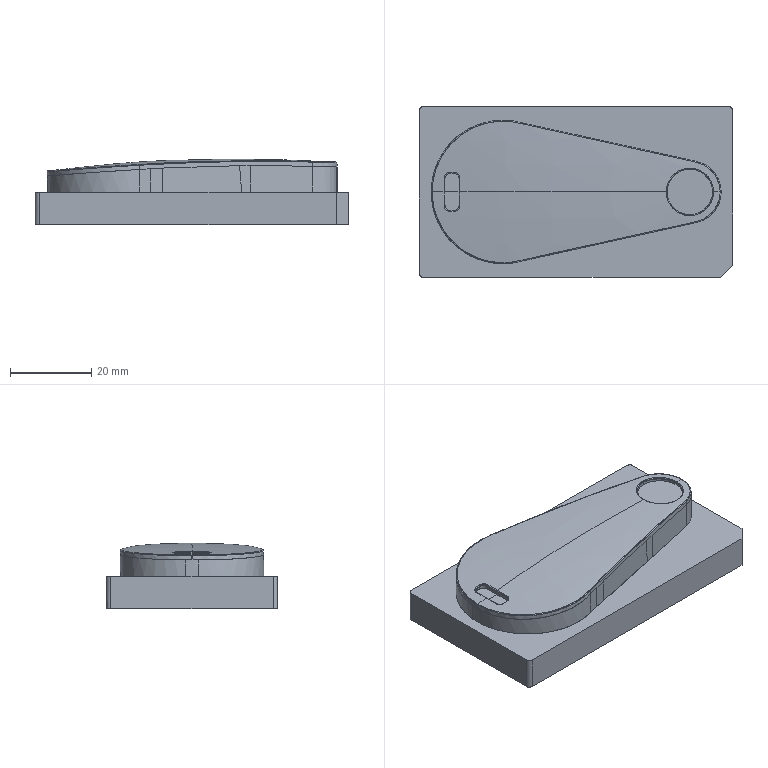NC program | PowerMill | posted with a generic post | part box 77 x 42 x 16.114 mm
Lines 19133 to 19848 of 230441:
N19230 M6
N19231 S18000 M03
N19232 G00 G90 X0.0 Y0.0
N19233 G43 Z10.803 H7
N19234
N19235 G05 P10000 R8
N19236 X35.209 Y-6.2591
N19237 Z-1.6006
N19238 G01 Z-2.8006 F1200.0
N19239 X35.1832 Y-6.2849 Z-2.7731 F2000.0
N19240 X35.1632 Y-6.3049 Z-2.7589
N19241 X35.1188 Y-6.3493 Z-2.7306
N19242 X35.0729 Y-6.3952 Z-2.7057
N19243 X35.0249 Y-6.4432 Z-2.6838
N19244 X34.9746 Y-6.4935 Z-2.6649
N19245 X34.9217 Y-6.5464 Z-2.6492
N19246 X34.8658 Y-6.6023 Z-2.6366
N19247 X34.8065 Y-6.6616 Z-2.6271
N19248 X34.772 Y-6.6961 Z-2.6234
N19249 X34.7334 Y-6.7347 Z-2.6213
N19250 X34.6899 Y-6.7782 Z-2.6212
N19251 X34.641 Y-6.8271 Z-2.6235
N19252 X34.5867 Y-6.8814 Z-2.6292
N19253 X34.5286 Y-6.9395 Z-2.6389
N19254 X34.4736 Y-6.9945 Z-2.6518
N19255 X34.4234 Y-7.0447 Z-2.6671
N19256 X34.3781 Y-7.09 Z-2.6843
N19257 X34.3373 Y-7.1308 Z-2.7032
N19258 X34.3008 Y-7.1673 Z-2.7235
N19259 X34.2682 Y-7.1999 Z-2.7452
N19260 X34.2385 Y-7.2296 Z-2.7686
N19261 X34.2146 Y-7.2535 Z-2.7954
N19262 X33.8245 Y-7.5729 Z-2.7981
N19263 X33.8519 Y-7.5454 Z-2.7464
N19264 X33.8774 Y-7.52 Z-2.7145
N19265 X33.9039 Y-7.4935 Z-2.6845
N19266 X33.9315 Y-7.4659 Z-2.6565
N19267 X33.9608 Y-7.4366 Z-2.6306
N19268 X33.9951 Y-7.4023 Z-2.6044
N19269 X34.031 Y-7.3663 Z-2.5806
N19270 X34.0646 Y-7.3327 Z-2.5605
N19271 X34.0976 Y-7.2998 Z-2.5418
N19272 X34.1447 Y-7.2527 Z-2.5181
N19273 X34.1959 Y-7.2015 Z-2.4964
N19274 X34.2517 Y-7.1457 Z-2.4768
N19275 X34.3126 Y-7.0848 Z-2.4593
N19276 X34.3735 Y-7.0238 Z-2.4452
N19277 X34.4416 Y-6.9558 Z-2.4327
N19278 X34.5099 Y-6.8875 Z-2.4237
N19279 X34.5798 Y-6.8176 Z-2.4182
N19280 X34.6486 Y-6.7487 Z-2.4166
N19281 X34.7173 Y-6.6801 Z-2.4183
N19282 X34.7812 Y-6.6162 Z-2.4228
N19283 X34.8542 Y-6.5432 Z-2.4313
N19284 X34.9245 Y-6.4729 Z-2.4434
N19285 X34.9922 Y-6.4052 Z-2.4588
N19286 X35.0574 Y-6.34 Z-2.4775
N19287 X35.1203 Y-6.2771 Z-2.4995
N19288 X35.1767 Y-6.2207 Z-2.5227
N19289 X35.2302 Y-6.1672 Z-2.5473
N19290 X35.2794 Y-6.1179 Z-2.5733
N19291 X35.3244 Y-6.073 Z-2.6006
N19292 X35.3656 Y-6.0318 Z-2.6297
N19293 X35.4036 Y-5.9938 Z-2.6606
N19294 X35.439 Y-5.9584 Z-2.6936
N19295 X35.4722 Y-5.9251 Z-2.7287
N19296 X35.5037 Y-5.8937 Z-2.7662
N19297 X35.5144 Y-5.8829 Z-2.78
N19298 X35.5428 Y-5.8546 Z-2.8245
N19299 X35.7727 Y-5.554 Z-2.8919
N19300 X35.7671 Y-5.5595 Z-2.869
N19301 X35.7378 Y-5.5889 Z-2.8034
N19302 X35.6641 Y-5.6625 Z-2.6896
N19303 X35.6342 Y-5.6924 Z-2.6536
N19304 X35.6006 Y-5.726 Z-2.6181
N19305 X35.563 Y-5.7637 Z-2.583
N19306 X35.5208 Y-5.8058 Z-2.5483
N19307 X35.4739 Y-5.8527 Z-2.5139
N19308 X35.4221 Y-5.9046 Z-2.4803
N19309 X35.366 Y-5.9607 Z-2.4481
N19310 X35.3094 Y-6.0173 Z-2.4194
N19311 X35.2572 Y-6.0695 Z-2.3958
N19312 X35.2101 Y-6.1165 Z-2.3768
N19313 X35.1703 Y-6.1564 Z-2.3621
N19314 X35.1015 Y-6.2252 Z-2.3394
N19315 X35.0322 Y-6.2944 Z-2.32
N19316 X34.96 Y-6.3667 Z-2.3036
N19317 X34.8838 Y-6.4429 Z-2.2902
N19318 X34.8112 Y-6.5155 Z-2.2807
N19319 X34.7406 Y-6.586 Z-2.274
N19320 X34.6712 Y-6.6555 Z-2.2698
N19321 X34.595 Y-6.7316 Z-2.2685
N19322 X34.5156 Y-6.8111 Z-2.2706
N19323 X34.4341 Y-6.8925 Z-2.2766
N19324 X34.3538 Y-6.9729 Z-2.2864
N19325 X34.2759 Y-7.0508 Z-2.2998
N19326 X34.2013 Y-7.1254 Z-2.3163
N19327 X34.1305 Y-7.1962 Z-2.3358
N19328 X34.0636 Y-7.2631 Z-2.3579
N19329 X34.0006 Y-7.3261 Z-2.3823
N19330 X33.945 Y-7.3817 Z-2.4072
N19331 X33.891 Y-7.4357 Z-2.4348
N19332 X33.8399 Y-7.4867 Z-2.4647
N19333 X33.7928 Y-7.5339 Z-2.4961
N19334 X33.7497 Y-7.577 Z-2.5289
N19335 X33.7105 Y-7.6162 Z-2.5628
N19336 X33.6749 Y-7.6518 Z-2.5979
N19337 X33.6427 Y-7.6839 Z-2.6341
N19338 X33.6138 Y-7.7128 Z-2.6714
N19339 X33.588 Y-7.7387 Z-2.7098
N19340 X33.5651 Y-7.7615 Z-2.7493
N19341 X33.5505 Y-7.7762 Z-2.7859
N19342 X33.3282 Y-7.9277 Z-2.7558
N19343 X33.3408 Y-7.9152 Z-2.7223
N19344 X33.3633 Y-7.8926 Z-2.6797
N19345 X33.3886 Y-7.8674 Z-2.6386
N19346 X33.4167 Y-7.8393 Z-2.5987
N19347 X33.4479 Y-7.808 Z-2.56
N19348 X33.4825 Y-7.7735 Z-2.5224
N19349 X33.5206 Y-7.7354 Z-2.4857
N19350 X33.5627 Y-7.6933 Z-2.45
N19351 X33.6092 Y-7.6468 Z-2.415
N19352 X33.6606 Y-7.5953 Z-2.3806
N19353 X33.7174 Y-7.5385 Z-2.3466
N19354 X33.7775 Y-7.4785 Z-2.3146
N19355 X33.8406 Y-7.4154 Z-2.2852
N19356 X33.907 Y-7.349 Z-2.2584
N19357 X33.977 Y-7.2789 Z-2.2342
N19358 X34.0511 Y-7.2049 Z-2.2127
N19359 X34.1295 Y-7.1264 Z-2.1938
N19360 X34.213 Y-7.043 Z-2.1776
N19361 X34.2918 Y-6.9641 Z-2.1656
N19362 X34.3796 Y-6.8764 Z-2.1558
N19363 X34.4683 Y-6.7876 Z-2.1498
N19364 X34.5585 Y-6.6975 Z-2.1477
N19365 X34.6495 Y-6.6065 Z-2.1495
N19366 X34.7407 Y-6.5152 Z-2.1553
N19367 X34.8312 Y-6.4247 Z-2.1651
N19368 X34.9205 Y-6.3355 Z-2.1787
N19369 X35.008 Y-6.248 Z-2.1959
N19370 X35.0933 Y-6.1627 Z-2.2165
N19371 X35.1734 Y-6.0826 Z-2.2396
N19372 X35.2491 Y-6.0069 Z-2.2652
N19373 X35.3208 Y-5.9351 Z-2.2934
N19374 X35.389 Y-5.8669 Z-2.324
N19375 X35.4514 Y-5.8045 Z-2.3558
N19376 X35.4908 Y-5.7652 Z-2.3781
N19377 X35.5297 Y-5.7263 Z-2.4018
N19378 X35.5682 Y-5.6878 Z-2.4268
N19379 X35.6062 Y-5.6498 Z-2.4534
N19380 X35.6414 Y-5.6146 Z-2.4805
N19381 X35.6858 Y-5.5701 Z-2.5182
N19382 X35.7265 Y-5.5295 Z-2.5564
N19383 X35.7633 Y-5.4927 Z-2.5952
N19384 X35.7966 Y-5.4594 Z-2.6349
N19385 X35.8267 Y-5.4292 Z-2.6758
N19386 X35.8542 Y-5.4017 Z-2.718
N19387 X35.8755 Y-5.3805 Z-2.7547
N19388 X35.8939 Y-5.3621 Z-2.7906
N19389 X35.9099 Y-5.3461 Z-2.8287
N19390 X35.9234 Y-5.3325 Z-2.8686
N19391 X35.9275 Y-5.3285 Z-2.8826
N19392 X36.0575 Y-5.1277 Z-2.8765
N19393 X36.0572 Y-5.128 Z-2.8753
N19394 X36.0477 Y-5.1376 Z-2.8412
N19395 X36.0344 Y-5.1509 Z-2.8038
N19396 X36.0227 Y-5.1625 Z-2.7755
N19397 X36.0098 Y-5.1755 Z-2.7484
N19398 X35.9959 Y-5.1894 Z-2.7223
N19399 X35.9738 Y-5.2114 Z-2.6842
N19400 X35.9562 Y-5.2291 Z-2.6556
N19401 X35.9404 Y-5.2448 Z-2.6316
N19402 X35.924 Y-5.2613 Z-2.6085
N19403 X35.8868 Y-5.2984 Z-2.5626
N19404 X35.8466 Y-5.3386 Z-2.5182
N19405 X35.8035 Y-5.3817 Z-2.4755
N19406 X35.7572 Y-5.428 Z-2.4344
N19407 X35.7074 Y-5.4779 Z-2.3947
N19408 X35.6535 Y-5.5318 Z-2.3563
N19409 X35.5948 Y-5.5904 Z-2.3188
N19410 X35.5303 Y-5.6549 Z-2.2818
N19411 X35.4676 Y-5.7176 Z-2.2492
N19412 X35.3998 Y-5.7854 Z-2.2177
N19413 X35.3296 Y-5.8557 Z-2.1888
N19414 X35.2541 Y-5.9312 Z-2.1616
N19415 X35.1731 Y-6.0121 Z-2.1361
N19416 X35.0868 Y-6.0984 Z-2.1129
N19417 X34.9959 Y-6.1894 Z-2.0924
N19418 X34.9021 Y-6.2831 Z-2.0752
N19419 X34.8109 Y-6.3744 Z-2.0622
N19420 X34.7245 Y-6.4607 Z-2.0531
N19421 X34.6439 Y-6.5413 Z-2.0474
N19422 X34.5729 Y-6.6123 Z-2.0448
N19423 X34.502 Y-6.6833 Z-2.0445
N19424 X34.431 Y-6.7543 Z-2.0463
N19425 X34.343 Y-6.8423 Z-2.051
N19426 X34.2721 Y-6.9131 Z-2.0569
N19427 X34.2014 Y-6.9838 Z-2.065
N19428 X34.1309 Y-7.0544 Z-2.0758
N19429 X34.0468 Y-7.1384 Z-2.0922
N19430 X33.9599 Y-7.2254 Z-2.1124
N19431 X33.8792 Y-7.306 Z-2.1348
N19432 X33.8035 Y-7.3817 Z-2.1596
N19433 X33.732 Y-7.4533 Z-2.1868
N19434 X33.6635 Y-7.5218 Z-2.2167
N19435 X33.6234 Y-7.5618 Z-2.2362
N19436 X33.5782 Y-7.607 Z-2.2602
N19437 X33.525 Y-7.6603 Z-2.2913
N19438 X33.4676 Y-7.7176 Z-2.3283
N19439 X33.4199 Y-7.7653 Z-2.3624
N19440 X33.38 Y-7.8052 Z-2.3938
N19441 X33.3463 Y-7.8389 Z-2.4231
N19442 X33.3144 Y-7.8709 Z-2.454
N19443 X33.2883 Y-7.897 Z-2.4821
N19444 X33.2625 Y-7.9228 Z-2.5111
N19445 X33.2357 Y-7.9495 Z-2.5434
N19446 X33.2086 Y-7.9767 Z-2.5802
N19447 X33.1863 Y-7.9989 Z-2.6149
N19448 X33.1659 Y-8.0193 Z-2.6511
N19449 X33.1471 Y-8.0381 Z-2.6889
N19450 X33.1296 Y-8.0556 Z-2.7281
N19451 X33.1238 Y-8.0615 Z-2.742
N19452 X33.1196 Y-8.0657 Z-2.757
N19453 X32.9272 Y-8.1873 Z-2.7697
N19454 X32.9407 Y-8.1739 Z-2.7281
N19455 X32.9561 Y-8.1585 Z-2.6877
N19456 X32.974 Y-8.1405 Z-2.6476
N19457 X32.9951 Y-8.1194 Z-2.6072
N19458 X33.0202 Y-8.0943 Z-2.5656
N19459 X33.0498 Y-8.0648 Z-2.5223
N19460 X33.0737 Y-8.0408 Z-2.4898
N19461 X33.1033 Y-8.0112 Z-2.4531
N19462 X33.1357 Y-7.9788 Z-2.4175
N19463 X33.1733 Y-7.9412 Z-2.3804
N19464 X33.2168 Y-7.8977 Z-2.3418
N19465 X33.2669 Y-7.8476 Z-2.3016
N19466 X33.3216 Y-7.793 Z-2.262
N19467 X33.3712 Y-7.7433 Z-2.2294
N19468 X33.4168 Y-7.6978 Z-2.2021
N19469 X33.4764 Y-7.6381 Z-2.1698
N19470 X33.5384 Y-7.5761 Z-2.1398
N19471 X33.6085 Y-7.506 Z-2.1095
N19472 X33.6863 Y-7.4282 Z-2.0799
N19473 X33.7616 Y-7.353 Z-2.0548
N19474 X33.8289 Y-7.2856 Z-2.0352
N19475 X33.8918 Y-7.2227 Z-2.0193
N19476 X33.9852 Y-7.1293 Z-1.9992
N19477 X34.0813 Y-7.0333 Z-1.9826
N19478 X34.1796 Y-6.9349 Z-1.9695
N19479 X34.2796 Y-6.8349 Z-1.9602
N19480 X34.3807 Y-6.7338 Z-1.9547
N19481 X34.477 Y-6.6376 Z-1.9532
N19482 X34.5751 Y-6.5395 Z-1.9552
N19483 X34.6786 Y-6.436 Z-1.9609
N19484 X34.7808 Y-6.3338 Z-1.9705
N19485 X34.8777 Y-6.2368 Z-1.9832
N19486 X34.9549 Y-6.1596 Z-1.996
N19487 X35.0336 Y-6.081 Z-2.0117
N19488 X35.1185 Y-5.996 Z-2.0318
N19489 X35.2083 Y-5.9063 Z-2.0566
N19490 X35.2966 Y-5.8179 Z-2.0848
N19491 X35.3796 Y-5.735 Z-2.1151
N19492 X35.4563 Y-5.6582 Z-2.1467
N19493 X35.5269 Y-5.5877 Z-2.1793
N19494 X35.5942 Y-5.5204 Z-2.214
N19495 X35.6559 Y-5.4587 Z-2.2493
N19496 X35.7185 Y-5.396 Z-2.2888
N19497 X35.7757 Y-5.3389 Z-2.3287
N19498 X35.8282 Y-5.2863 Z-2.3695
N19499 X35.8768 Y-5.2377 Z-2.4114
N19500 X35.9098 Y-5.2047 Z-2.4427
N19501 X35.9428 Y-5.1717 Z-2.4765
N19502 X35.9832 Y-5.1313 Z-2.5216
N19503 X36.0133 Y-5.1012 Z-2.5583
N19504 X36.042 Y-5.0725 Z-2.597
N19505 X36.053 Y-5.0616 Z-2.6134
N19506 X36.0645 Y-5.05 Z-2.6318
N19507 X36.0817 Y-5.0328 Z-2.6605
N19508 X36.0945 Y-5.02 Z-2.6827
N19509 X36.1043 Y-5.0102 Z-2.7006
N19510 X36.1121 Y-5.0024 Z-2.716
N19511 X36.1358 Y-4.9787 Z-2.7691
N19512 X36.1514 Y-4.9631 Z-2.8077
N19513 X36.1625 Y-4.952 Z-2.8414
N19514 X36.1693 Y-4.9452 Z-2.8682
N19515 X36.2652 Y-4.7787 Z-2.8501
N19516 X36.2566 Y-4.7872 Z-2.8178
N19517 X36.2444 Y-4.7994 Z-2.782
N19518 X36.2276 Y-4.8163 Z-2.7409
N19519 X36.2021 Y-4.8417 Z-2.6847
N19520 X36.1971 Y-4.8468 Z-2.675
N19521 X36.1691 Y-4.8747 Z-2.6253
N19522 X36.1383 Y-4.9055 Z-2.5767
N19523 X36.1045 Y-4.9393 Z-2.5293
N19524 X36.0676 Y-4.9763 Z-2.4829
N19525 X36.0272 Y-5.0167 Z-2.4375
N19526 X35.9831 Y-5.0607 Z-2.393
N19527 X35.9351 Y-5.1088 Z-2.3492
N19528 X35.8826 Y-5.1613 Z-2.306
N19529 X35.8236 Y-5.2202 Z-2.2616
N19530 X35.7635 Y-5.2803 Z-2.2204
N19531 X35.6992 Y-5.3446 Z-2.1805
N19532 X35.6354 Y-5.4084 Z-2.145
N19533 X35.5725 Y-5.4713 Z-2.1133
N19534 X35.5089 Y-5.5349 Z-2.0841
N19535 X35.4244 Y-5.6194 Z-2.0488
N19536 X35.3392 Y-5.7046 Z-2.0172
N19537 X35.251 Y-5.7928 Z-1.9884
N19538 X35.1613 Y-5.8825 Z-1.9632
N19539 X35.0739 Y-5.97 Z-1.942
N19540 X34.9865 Y-6.0573 Z-1.9239
N19541 X34.88 Y-6.1638 Z-1.9054
N19542 X34.7729 Y-6.2709 Z-1.8909
N19543 X34.6654 Y-6.3784 Z-1.8804
N19544 X34.5576 Y-6.4863 Z-1.8738
N19545 X34.4494 Y-6.5944 Z-1.8713
N19546 X34.341 Y-6.7028 Z-1.8727
N19547 X34.2326 Y-6.8113 Z-1.8781
N19548 X34.1241 Y-6.9198 Z-1.8875
N19549 X34.022 Y-7.0218 Z-1.9
N19550 X33.9241 Y-7.1197 Z-1.9158
N19551 X33.83 Y-7.2138 Z-1.9348
N19552 X33.7394 Y-7.3044 Z-1.9569
N19553 X33.652 Y-7.3918 Z-1.9821
N19554 X33.5677 Y-7.4761 Z-2.0104
N19555 X33.4863 Y-7.5576 Z-2.0416
N19556 X33.4075 Y-7.6363 Z-2.0758
N19557 X33.339 Y-7.7048 Z-2.1092
N19558 X33.2733 Y-7.7705 Z-2.1453
N19559 X33.2121 Y-7.8318 Z-2.1828
N19560 X33.1558 Y-7.888 Z-2.2212
N19561 X33.103 Y-7.9408 Z-2.2611
N19562 X33.053 Y-7.9908 Z-2.3027
N19563 X33.0085 Y-8.0353 Z-2.3437
N19564 X32.969 Y-8.0749 Z-2.3843
N19565 X32.9338 Y-8.1101 Z-2.4249
N19566 X32.9025 Y-8.1413 Z-2.4655
N19567 X32.8738 Y-8.17 Z-2.5073
N19568 X32.8446 Y-8.1992 Z-2.5535
N19569 X32.82 Y-8.2238 Z-2.5973
N19570 X32.7994 Y-8.2444 Z-2.6396
N19571 X32.7821 Y-8.2617 Z-2.6813
N19572 X32.7675 Y-8.2763 Z-2.7232
N19573 X32.7551 Y-8.2887 Z-2.766
N19574 X32.5984 Y-8.3747 Z-2.7382
N19575 X32.6006 Y-8.3725 Z-2.73
N19576 X32.6164 Y-8.3567 Z-2.6835
N19577 X32.6337 Y-8.3394 Z-2.6381
N19578 X32.6528 Y-8.3203 Z-2.5942
N19579 X32.674 Y-8.2992 Z-2.5522
N19580 X32.6978 Y-8.2753 Z-2.5109
N19581 X32.7224 Y-8.2507 Z-2.4728
N19582 X32.7481 Y-8.225 Z-2.436
N19583 X32.7747 Y-8.1984 Z-2.4007
N19584 X32.8104 Y-8.1627 Z-2.3581
N19585 X32.8503 Y-8.1228 Z-2.3154
N19586 X32.8952 Y-8.0779 Z-2.2723
N19587 X32.9459 Y-8.0272 Z-2.2282
N19588 X32.9914 Y-7.9817 Z-2.1917
N19589 X33.0423 Y-7.9308 Z-2.1545
N19590 X33.0971 Y-7.876 Z-2.1184
N19591 X33.1595 Y-7.8136 Z-2.0813
N19592 X33.2291 Y-7.744 Z-2.0441
N19593 X33.2954 Y-7.6777 Z-2.012
N19594 X33.3554 Y-7.6177 Z-1.9857
N19595 X33.4351 Y-7.538 Z-1.9543
N19596 X33.5173 Y-7.4559 Z-1.9257
N19597 X33.6041 Y-7.369 Z-1.8994
N19598 X33.6959 Y-7.2773 Z-1.8754
N19599 X33.7924 Y-7.1807 Z-1.8541
N19600 X33.8935 Y-7.0796 Z-1.8358
N19601 X33.9983 Y-6.9748 Z-1.8207
N19602 X34.1052 Y-6.8679 Z-1.8092
N19603 X34.2107 Y-6.7624 Z-1.8016
N19604 X34.3121 Y-6.661 Z-1.7976
N19605 X34.4081 Y-6.565 Z-1.7968
N19606 X34.516 Y-6.4571 Z-1.7992
N19607 X34.6239 Y-6.3493 Z-1.8052
N19608 X34.7316 Y-6.2416 Z-1.8149
N19609 X34.839 Y-6.1341 Z-1.8283
N19610 X34.9327 Y-6.0404 Z-1.8431
N19611 X35.0362 Y-5.9369 Z-1.8627
N19612 X35.1377 Y-5.8354 Z-1.8856
N19613 X35.2359 Y-5.7372 Z-1.9116
N19614 X35.3302 Y-5.6429 Z-1.9404
N19615 X35.4202 Y-5.5529 Z-1.9717
N19616 X35.5059 Y-5.4672 Z-2.0054
N19617 X35.5875 Y-5.3856 Z-2.0414
N19618 X35.665 Y-5.3081 Z-2.0794
N19619 X35.7387 Y-5.2344 Z-2.1196
N19620 X35.8086 Y-5.1645 Z-2.1617
N19621 X35.8712 Y-5.1019 Z-2.2031
N19622 X35.9298 Y-5.0433 Z-2.246
N19623 X35.9848 Y-4.9883 Z-2.2904
N19624 X36.0365 Y-4.9367 Z-2.3365
N19625 X36.0849 Y-4.8882 Z-2.3842
N19626 X36.1283 Y-4.8448 Z-2.4313
N19627 X36.1675 Y-4.8057 Z-2.4781
N19628 X36.2024 Y-4.7707 Z-2.5246
N19629 X36.2341 Y-4.739 Z-2.5719
N19630 X36.2574 Y-4.7157 Z-2.6104
N19631 X36.272 Y-4.7011 Z-2.6375
N19632 X36.2859 Y-4.6872 Z-2.6654
N19633 X36.2994 Y-4.6737 Z-2.6936
N19634 X36.3124 Y-4.6607 Z-2.7223
N19635 X36.3211 Y-4.652 Z-2.7429
N19636 X36.3347 Y-4.6384 Z-2.7766
N19637 X36.3458 Y-4.6273 Z-2.8122
N19638 X36.3507 Y-4.6224 Z-2.8317
N19639 X36.4344 Y-4.468 Z-2.8343
N19640 X36.4166 Y-4.4858 Z-2.774
N19641 X36.4142 Y-4.4882 Z-2.7669
N19642 X36.4048 Y-4.4976 Z-2.7422
N19643 X36.395 Y-4.5074 Z-2.7178
N19644 X36.3806 Y-4.5218 Z-2.6835
N19645 X36.37 Y-4.5324 Z-2.6597
N19646 X36.3589 Y-4.5435 Z-2.6365
N19647 X36.3324 Y-4.57 Z-2.5881
N19648 X36.302 Y-4.6004 Z-2.5388
N19649 X36.2673 Y-4.6351 Z-2.4885
N19650 X36.228 Y-4.6744 Z-2.4369
N19651 X36.1948 Y-4.7076 Z-2.3969
N19652 X36.1546 Y-4.7478 Z-2.3529
N19653 X36.1104 Y-4.792 Z-2.3092
N19654 X36.0662 Y-4.8362 Z-2.2689
N19655 X36.0227 Y-4.8797 Z-2.2317
N19656 X35.9713 Y-4.9311 Z-2.1915
N19657 X35.9161 Y-4.9863 Z-2.1519
N19658 X35.8527 Y-5.0497 Z-2.1102
N19659 X35.7808 Y-5.1216 Z-2.0672
N19660 X35.7118 Y-5.1906 Z-2.0295
N19661 X35.6508 Y-5.2517 Z-1.9988
N19662 X35.5949 Y-5.3075 Z-1.9731
N19663 X35.521 Y-5.3814 Z-1.9419
N19664 X35.4327 Y-5.4697 Z-1.9083
N19665 X35.3402 Y-5.5622 Z-1.8769
N19666 X35.2434 Y-5.659 Z-1.8479
N19667 X35.1423 Y-5.7601 Z-1.8215
N19668 X35.037 Y-5.8654 Z-1.7979
N19669 X34.9278 Y-5.9746 Z-1.7774
N19670 X34.8153 Y-6.0871 Z-1.7602
N19671 X34.7004 Y-6.202 Z-1.7466
N19672 X34.5844 Y-6.318 Z-1.7369
N19673 X34.4697 Y-6.4327 Z-1.731
N19674 X34.358 Y-6.5444 Z-1.7289
N19675 X34.2502 Y-6.6522 Z-1.7302
N19676 X34.1469 Y-6.7555 Z-1.7346
N19677 X34.0352 Y-6.8672 Z-1.7427
N19678 X33.9239 Y-6.9785 Z-1.7546
N19679 X33.817 Y-7.0854 Z-1.7697
N19680 X33.714 Y-7.1884 Z-1.788
N19681 X33.6146 Y-7.2878 Z-1.8096
N19682 X33.5184 Y-7.384 Z-1.8344
N19683 X33.4243 Y-7.4781 Z-1.8626
N19684 X33.3358 Y-7.5666 Z-1.8928
N19685 X33.2529 Y-7.6495 Z-1.9248
N19686 X33.1748 Y-7.7276 Z-1.9589
N19687 X33.1008 Y-7.8016 Z-1.9951
N19688 X33.0316 Y-7.8708 Z-2.0328
N19689 X32.9664 Y-7.936 Z-2.0724
N19690 X32.9049 Y-7.9976 Z-2.1139
N19691 X32.8466 Y-8.0557 Z-2.1573
N19692 X32.7916 Y-8.1108 Z-2.2026
N19693 X32.7394 Y-8.163 Z-2.25
N19694 X32.7038 Y-8.1986 Z-2.2856
N19695 X32.6625 Y-8.2399 Z-2.3308
N19696 X32.6243 Y-8.2781 Z-2.3774
N19697 X32.5895 Y-8.3129 Z-2.4249
N19698 X32.558 Y-8.3444 Z-2.473
N19699 X32.5298 Y-8.3726 Z-2.5216
N19700 X32.5048 Y-8.3976 Z-2.5705
N19701 X32.483 Y-8.4194 Z-2.6196
N19702 X32.4643 Y-8.4381 Z-2.6691
N19703 X32.4486 Y-8.4538 Z-2.7187
N19704 X32.4457 Y-8.4567 Z-2.7308
N19705 X32.2927 Y-8.539 Z-2.7592
N19706 X32.3001 Y-8.5316 Z-2.7219
N19707 X32.3147 Y-8.5169 Z-2.6715
N19708 X32.3323 Y-8.4994 Z-2.6212
N19709 X32.353 Y-8.4787 Z-2.5711
N19710 X32.3767 Y-8.455 Z-2.5213
N19711 X32.4037 Y-8.4279 Z-2.4716
N19712 X32.4341 Y-8.3976 Z-2.4221
N19713 X32.468 Y-8.3637 Z-2.373
N19714 X32.5053 Y-8.3264 Z-2.3244
N19715 X32.5462 Y-8.2855 Z-2.2764
N19716 X32.5903 Y-8.2414 Z-2.2297
N19717 X32.637 Y-8.1947 Z-2.1849
N19718 X32.6848 Y-8.1468 Z-2.1432
N19719 X32.7373 Y-8.0944 Z-2.1017
N19720 X32.7942 Y-8.0375 Z-2.0608
N19721 X32.8571 Y-7.9746 Z-2.0196
N19722 X32.9261 Y-7.9056 Z-1.9786
N19723 X33.0002 Y-7.8315 Z-1.9388
N19724 X33.0737 Y-7.758 Z-1.9031
N19725 X33.1422 Y-7.6895 Z-1.8731
N19726 X33.2007 Y-7.631 Z-1.8498
N19727 X33.2909 Y-7.5408 Z-1.8177
N19728 X33.3844 Y-7.4473 Z-1.7884
N19729 X33.4816 Y-7.3501 Z-1.762
N19730 X33.583 Y-7.2486 Z-1.7384
N19731 X33.6892 Y-7.1425 Z-1.7178
N19732 X33.7963 Y-7.0353 Z-1.7006
N19733 X33.909 Y-6.9227 Z-1.6864
N19734 X34.0221 Y-6.8096 Z-1.6759
N19735 X34.139 Y-6.6927 Z-1.6689
N19736 X34.259 Y-6.5727 Z-1.6656
N19737 X34.381 Y-6.4507 Z-1.6662
N19738 X34.5027 Y-6.329 Z-1.6708
N19739 X34.6222 Y-6.2095 Z-1.6791
N19740 X34.7383 Y-6.0934 Z-1.6909
N19741 X34.8509 Y-5.9808 Z-1.706
N19742 X34.9693 Y-5.8624 Z-1.7256
N19743 X35.0818 Y-5.7499 Z-1.7479
N19744 X35.1891 Y-5.6426 Z-1.773
N19745 X35.2918 Y-5.5399 Z-1.8009
N19746 X35.3904 Y-5.4413 Z-1.8315
N19747 X35.4853 Y-5.3464 Z-1.8648
N19748 X35.5768 Y-5.2549 Z-1.9009
N19749 X35.6618 Y-5.1699 Z-1.9382
N19750 X35.7429 Y-5.0888 Z-1.9776
N19751 X35.8195 Y-5.0122 Z-2.0188
N19752 X35.8917 Y-4.94 Z-2.0615
N19753 X35.9595 Y-4.8722 Z-2.1057
N19754 X36.0231 Y-4.8086 Z-2.1513
N19755 X36.0815 Y-4.7502 Z-2.1971
N19756 X36.1368 Y-4.6949 Z-2.2447
N19757 X36.188 Y-4.6437 Z-2.2931
N19758 X36.2353 Y-4.5963 Z-2.3424
N19759 X36.2791 Y-4.5525 Z-2.3926
N19760 X36.3196 Y-4.5121 Z-2.4439
N19761 X36.3569 Y-4.4748 Z-2.4962
N19762 X36.3912 Y-4.4405 Z-2.5497
N19763 X36.4071 Y-4.4246 Z-2.5773
N19764 X36.4221 Y-4.4095 Z-2.6061
N19765 X36.4365 Y-4.3952 Z-2.6355
N19766 X36.4522 Y-4.3795 Z-2.6698
N19767 X36.4711 Y-4.3606 Z-2.7149
N19768 X36.4888 Y-4.3429 Z-2.7624
N19769 X36.5013 Y-4.3304 Z-2.8016
N19770 X36.51 Y-4.3217 Z-2.8347
N19771 X36.5136 Y-4.3181 Z-2.8517
N19772 X36.5864 Y-4.1746 Z-2.8726
N19773 X36.5821 Y-4.1789 Z-2.8466
N19774 X36.5747 Y-4.1863 Z-2.8145
N19775 X36.5642 Y-4.1968 Z-2.778
N19776 X36.55 Y-4.211 Z-2.7362
N19777 X36.5311 Y-4.2299 Z-2.6875
N19778 X36.5061 Y-4.2549 Z-2.6308
N19779 X36.4834 Y-4.2776 Z-2.5843
N19780 X36.4639 Y-4.2971 Z-2.5474
N19781 X36.447 Y-4.314 Z-2.5177
N19782 X36.4319 Y-4.3291 Z-2.4933
N19783 X36.4163 Y-4.3447 Z-2.4697
N19784 X36.3783 Y-4.3826 Z-2.4169
N19785 X36.3371 Y-4.4239 Z-2.3649
N19786 X36.2923 Y-4.4687 Z-2.3136
N19787 X36.2438 Y-4.5172 Z-2.2632
N19788 X36.1915 Y-4.5695 Z-2.2136
N19789 X36.1352 Y-4.6258 Z-2.1649
N19790 X36.0746 Y-4.6863 Z-2.1172
N19791 X36.0099 Y-4.7511 Z-2.0705
N19792 X35.941 Y-4.82 Z-2.0253
N19793 X35.8687 Y-4.8923 Z-1.982
N19794 X35.7944 Y-4.9666 Z-1.9414
N19795 X35.7226 Y-5.0383 Z-1.9055
N19796 X35.6414 Y-5.1196 Z-1.8687
N19797 X35.5595 Y-5.2015 Z-1.835
N19798 X35.4683 Y-5.2927 Z-1.8013
N19799 X35.3684 Y-5.3926 Z-1.7682
N19800 X35.2648 Y-5.4961 Z-1.7377
N19801 X35.169 Y-5.592 Z-1.7128
N19802 X35.0821 Y-5.6789 Z-1.6928
N19803 X34.9976 Y-5.7634 Z-1.6757
N19804 X34.8809 Y-5.8801 Z-1.6554
N19805 X34.7615 Y-5.9994 Z-1.6385
N19806 X34.6386 Y-6.1223 Z-1.625
N19807 X34.5131 Y-6.2478 Z-1.6152
N19808 X34.3862 Y-6.3748 Z-1.6093
N19809 X34.26 Y-6.5009 Z-1.6073
N19810 X34.1363 Y-6.6247 Z-1.6092
N19811 X34.016 Y-6.745 Z-1.6146
N19812 X33.8969 Y-6.8641 Z-1.6237
N19813 X33.7794 Y-6.9816 Z-1.6364
N19814 X33.6659 Y-7.0951 Z-1.6524
N19815 X33.556 Y-7.205 Z-1.6718
N19816 X33.4495 Y-7.3115 Z-1.6945
N19817 X33.3457 Y-7.4153 Z-1.7204
N19818 X33.2488 Y-7.5122 Z-1.7483
N19819 X33.1575 Y-7.6034 Z-1.7784
N19820 X33.0711 Y-7.6899 Z-1.8107
N19821 X32.9922 Y-7.7688 Z-1.8438
N19822 X32.9142 Y-7.8468 Z-1.8801
N19823 X32.839 Y-7.9219 Z-1.919
N19824 X32.7679 Y-7.9931 Z-1.9597
N19825 X32.7011 Y-8.0599 Z-2.0019
N19826 X32.6388 Y-8.1222 Z-2.0453
N19827 X32.5807 Y-8.1803 Z-2.0899
N19828 X32.5267 Y-8.2343 Z-2.1356
N19829 X32.4765 Y-8.2845 Z-2.1823
N19830 X32.43 Y-8.331 Z-2.2301
N19831 X32.387 Y-8.374 Z-2.2789
N19832 X32.3474 Y-8.4136 Z-2.3286
N19833 X32.3238 Y-8.4372 Z-2.3612
N19834 X32.295 Y-8.466 Z-2.4048
N19835 X32.2657 Y-8.4952 Z-2.4542
N19836 X32.2381 Y-8.5229 Z-2.5065
N19837 X32.2138 Y-8.5472 Z-2.5587
N19838 X32.1932 Y-8.5678 Z-2.6096
N19839 X32.1762 Y-8.5848 Z-2.6587
N19840 X32.1627 Y-8.5983 Z-2.7059
N19841 X32.1525 Y-8.6085 Z-2.751
N19842 X32.1453 Y-8.6157 Z-2.7942
N19843 X32.0117 Y-8.6786 Z-2.7861
N19844 X32.0186 Y-8.6717 Z-2.7427
N19845 X32.0285 Y-8.6618 Z-2.6978
N19846 X32.0417 Y-8.6486 Z-2.6511
N19847 X32.0585 Y-8.6317 Z-2.6017
N19848 X32.0795 Y-8.6108 Z-2.5488
N19849 X32.1035 Y-8.5868 Z-2.4953
N19850 X32.1299 Y-8.5604 Z-2.4434
N19851 X32.1592 Y-8.531 Z-2.3924
N19852 X32.1917 Y-8.4985 Z-2.3421
N19853 X32.2276 Y-8.4627 Z-2.2925
N19854 X32.2669 Y-8.4234 Z-2.2435
N19855 X32.3101 Y-8.3802 Z-2.195
N19856 X32.3539 Y-8.3363 Z-2.1501
N19857 X32.403 Y-8.2873 Z-2.1044
N19858 X32.454 Y-8.2363 Z-2.061
N19859 X32.5113 Y-8.179 Z-2.0163
N19860 X32.5752 Y-8.1151 Z-1.9707
N19861 X32.6436 Y-8.0466 Z-1.9263
N19862 X32.7081 Y-7.9821 Z-1.8881
N19863 X32.767 Y-7.9232 Z-1.8562
N19864 X32.8232 Y-7.867 Z-1.8283
N19865 X32.9064 Y-7.7839 Z-1.7907
N19866 X32.9936 Y-7.6967 Z-1.7554
N19867 X33.0853 Y-7.605 Z-1.7223
N19868 X33.1821 Y-7.5082 Z-1.6914
N19869 X33.282 Y-7.4083 Z-1.6635
N19870 X33.3855 Y-7.3047 Z-1.6386
N19871 X33.4933 Y-7.197 Z-1.6166
N19872 X33.6057 Y-7.0845 Z-1.5977
N19873 X33.7236 Y-6.9666 Z-1.5818
N19874 X33.848 Y-6.8423 Z-1.5689
N19875 X33.9762 Y-6.7141 Z-1.5595
N19876 X34.1049 Y-6.5853 Z-1.5541
N19877 X34.2343 Y-6.456 Z-1.5527
N19878 X34.364 Y-6.3262 Z-1.5552
N19879 X34.4943 Y-6.196 Z-1.5617
N19880 X34.6195 Y-6.0708 Z-1.5718
N19881 X34.7441 Y-5.9462 Z-1.5854
N19882 X34.8676 Y-5.8227 Z-1.6025
N19883 X34.9883 Y-5.702 Z-1.6231
N19884 X35.1053 Y-5.585 Z-1.6468
N19885 X35.2179 Y-5.4724 Z-1.6735
N19886 X35.326 Y-5.3642 Z-1.7029
N19887 X35.4296 Y-5.2607 Z-1.7349
N19888 X35.5287 Y-5.1615 Z-1.7694
N19889 X35.6236 Y-5.0667 Z-1.8062
N19890 X35.7134 Y-4.9769 Z-1.8449
N19891 X35.7982 Y-4.8921 Z-1.8852
N19892 X35.8783 Y-4.812 Z-1.9272
N19893 X35.9539 Y-4.7363 Z-1.9709
N19894 X36.0254 Y-4.6648 Z-2.0162
N19895 X36.093 Y-4.5973 Z-2.0632
N19896 X36.1569 Y-4.5334 Z-2.1118
N19897 X36.2173 Y-4.473 Z-2.1621
N19898 X36.2707 Y-4.4196 Z-2.2107
N19899 X36.3207 Y-4.3696 Z-2.2606
N19900 X36.3673 Y-4.323 Z-2.3118
N19901 X36.4107 Y-4.2796 Z-2.3644
N19902 X36.4511 Y-4.2392 Z-2.4182
N19903 X36.4843 Y-4.206 Z-2.467
N19904 X36.516 Y-4.1743 Z-2.5185
N19905 X36.5452 Y-4.1451 Z-2.5715
N19906 X36.5713 Y-4.119 Z-2.6249
N19907 X36.5941 Y-4.0961 Z-2.6782
N19908 X36.6136 Y-4.0766 Z-2.7308
N19909 X36.6299 Y-4.0604 Z-2.7827
N19910 X36.6429 Y-4.0473 Z-2.8338
N19911 X36.6484 Y-4.0419 Z-2.8593
N19912 X36.7033 Y-3.9163 Z-2.8397
N19913 X36.7014 Y-3.9182 Z-2.8308
N19914 X36.6877 Y-3.9319 Z-2.7768
N19915 X36.6711 Y-3.9485 Z-2.7227
N19916 X36.6514 Y-3.9682 Z-2.6685
N19917 X36.6286 Y-3.991 Z-2.6143
N19918 X36.6025 Y-4.0171 Z-2.5601
N19919 X36.5731 Y-4.0465 Z-2.5059
N19920 X36.5403 Y-4.0793 Z-2.4518
N19921 X36.504 Y-4.1156 Z-2.398
N19922 X36.4643 Y-4.1553 Z-2.3448
N19923 X36.4215 Y-4.1981 Z-2.2926
N19924 X36.3761 Y-4.2434 Z-2.2423
N19925 X36.3248 Y-4.2948 Z-2.1903
N19926 X36.2696 Y-4.35 Z-2.1391
N19927 X36.2109 Y-4.4087 Z-2.0894
N19928 X36.1484 Y-4.4712 Z-2.0411
N19929 X36.0816 Y-4.5379 Z-1.9939
N19930 X36.0101 Y-4.6094 Z-1.9477
N19931 X35.9331 Y-4.6865 Z-1.9021
N19932 X35.8523 Y-4.7672 Z-1.8586
N19933 X35.7676 Y-4.8519 Z-1.817
N19934 X35.6784 Y-4.9411 Z-1.7774
N19935 X35.5845 Y-5.0351 Z-1.7397
N19936 X35.4857 Y-5.1339 Z-1.7042
N19937 X35.3819 Y-5.2376 Z-1.6709
N19938 X35.2736 Y-5.346 Z-1.6401
N19939 X35.1616 Y-5.458 Z-1.6121
N19940 X35.0476 Y-5.5719 Z-1.5873
N19941 X34.924 Y-5.6956 Z-1.5642
N19942 X34.7978 Y-5.8218 Z-1.5447
N19943 X34.6689 Y-5.9507 Z-1.5287
N19944 X34.5372 Y-6.0824 Z-1.5164
N19945 X34.4013 Y-6.2182 Z-1.5076